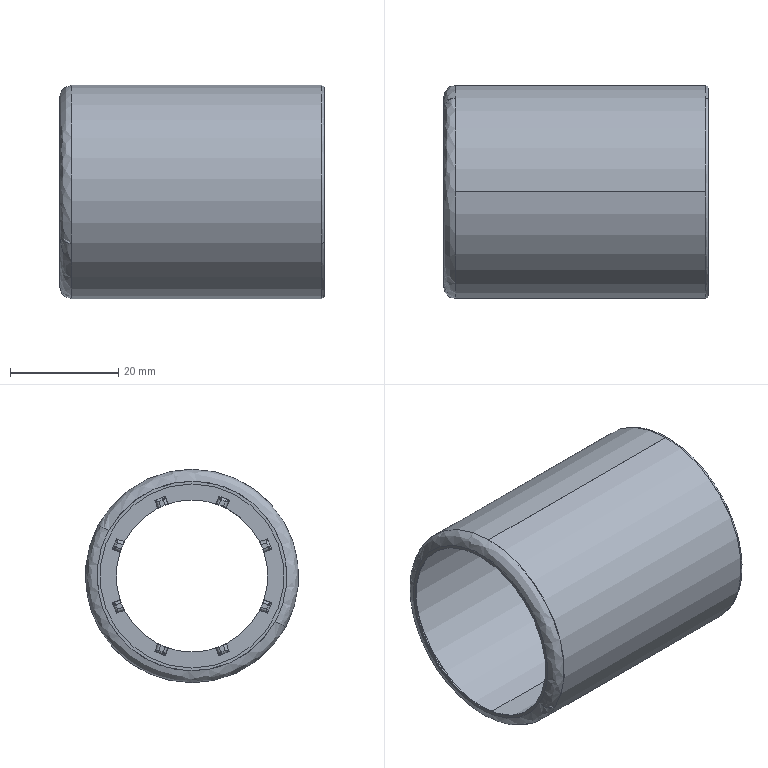Part | STEP file | TQ-DD-1105-THRotor cover1010_デフォルト | 1 solid | 242 faces | box 48.9 x 39.4 x 39.4 mm | volume 1331 mm3 | cylinder 116 | spline 74 | plane 52 | commonest cylinder face diameters 0.6 x55 0.2 x21 1 x16 30.6 x8 31 x8 28 x2